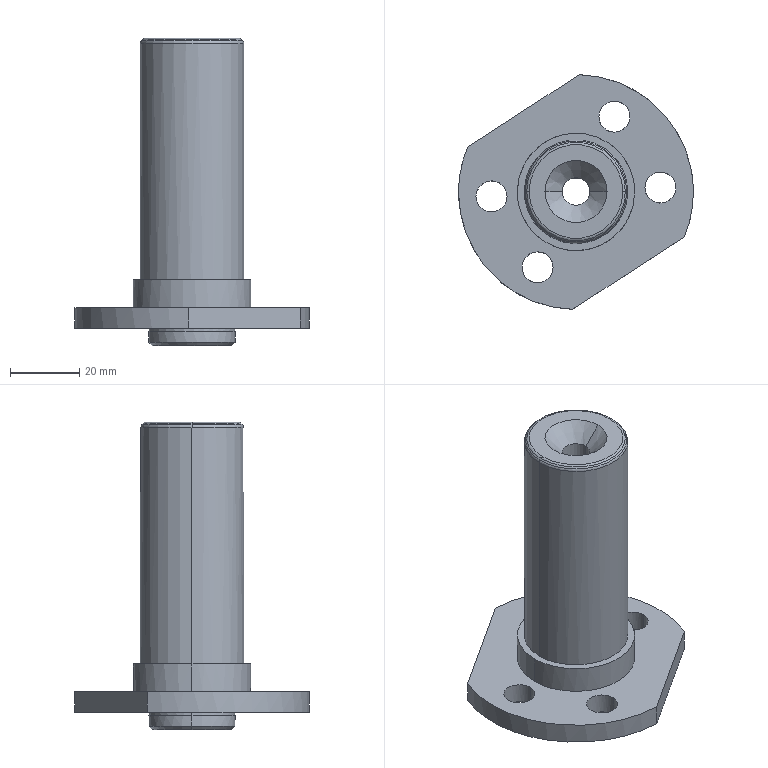Part | STEP file | Corpo da Bucha Acopladora - GRANDE | 1 solid | 43 faces | box 68 x 67.975 x 89.05 mm | volume 70986 mm3 | cylinder 23 | cone 8 | plane 8 | torus 4 | commonest cylinder face diameters 9 x8 68 x3 8 x2 12 x2 24.8 x2 25 x2